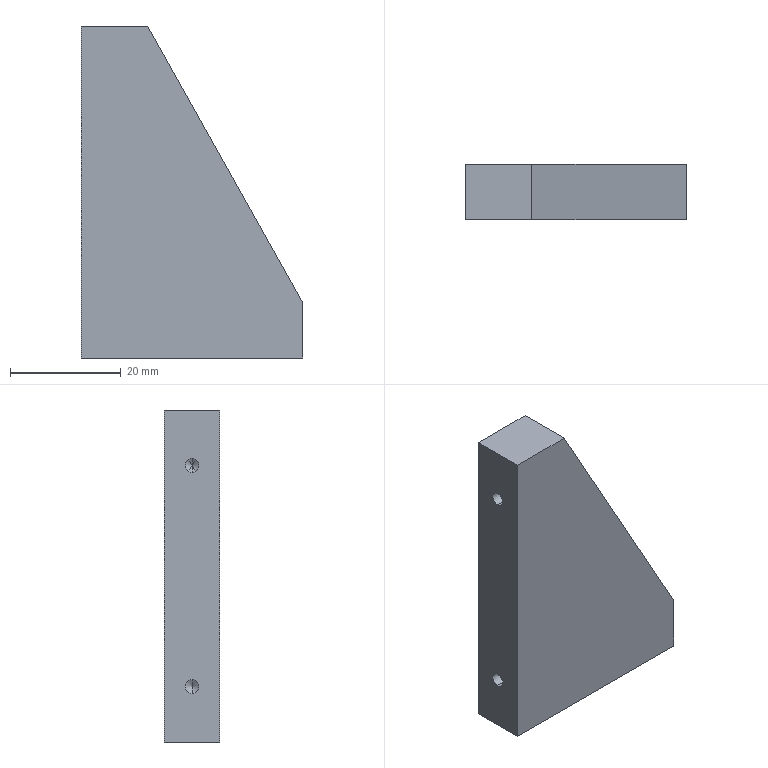Part | STEP file | PN_0031 | 1 solid | 19 faces | box 40 x 10 x 60 mm | volume 16813 mm3 | plane 7 | cylinder 6 | cone 6 | commonest cylinder face diameters 2.5 x4 3.3 x2
STEP:
#1=CARTESIAN_POINT('',(0.,0.,0.));
#2=DIRECTION('',(0.,0.,1.));
#3=DIRECTION('',(1.,0.,0.));
#4=AXIS2_PLACEMENT_3D('',#1,#2,#3);
#5=CARTESIAN_POINT('',(-1.65,5.,-18.5));
#6=VERTEX_POINT('',#5);
#7=CARTESIAN_POINT('',(-1.65,5.,-30.));
#8=VERTEX_POINT('',#7);
#9=CARTESIAN_POINT('',(-1.65,5.,-30.));
#10=DIRECTION('',(0.,0.,-1.));
#11=VECTOR('',#10,1.);
#12=LINE('',#9,#11);
#13=CARTESIAN_POINT('',(0.,5.,-30.));
#14=DIRECTION('',(0.,0.,-1.));
#15=DIRECTION('',(-1.,0.,0.));
#16=AXIS2_PLACEMENT_3D('',#13,#14,#15);
#17=CYLINDRICAL_SURFACE('',#16,1.65);
#18=CARTESIAN_POINT('',(6.283,0.));
#19=DIRECTION('',(0.,1.));
#20=VECTOR('',#19,1.);
#21=LINE('',#18,#20);
#22=(GEOMETRIC_REPRESENTATION_CONTEXT(2)PARAMETRIC_REPRESENTATION_CONTEXT()REPRESENTATION_CONTEXT('',''));
#23=DEFINITIONAL_REPRESENTATION('',(#21),#22);
#24=PCURVE('',#17,#23);
#25=CARTESIAN_POINT('',(0.,5.,-30.));
#26=DIRECTION('',(0.,0.,-1.));
#27=DIRECTION('',(-1.,0.,0.));
#28=AXIS2_PLACEMENT_3D('',#25,#26,#27);
#29=CYLINDRICAL_SURFACE('',#28,1.65);
#30=CARTESIAN_POINT('',(0.,0.));
#31=DIRECTION('',(0.,1.));
#32=VECTOR('',#31,1.);
#33=LINE('',#30,#32);
#34=(GEOMETRIC_REPRESENTATION_CONTEXT(2)PARAMETRIC_REPRESENTATION_CONTEXT()REPRESENTATION_CONTEXT('',''));
#35=DEFINITIONAL_REPRESENTATION('',(#33),#34);
#36=PCURVE('',#29,#35);
#37=SURFACE_CURVE('',#12,(#24,#36),.PCURVE_S1.);
#38=EDGE_CURVE('',#6,#8,#37,.T.);
#39=ORIENTED_EDGE('',*,*,#38,.T.);
#40=CARTESIAN_POINT('',(1.65,5.,-30.));
#41=VERTEX_POINT('',#40);
#42=CARTESIAN_POINT('',(0.,5.,-30.));
#43=DIRECTION('',(0.,0.,-1.));
#44=DIRECTION('',(-1.,0.,0.));
#45=AXIS2_PLACEMENT_3D('',#42,#43,#44);
#46=CIRCLE('',#45,1.65);
#47=CARTESIAN_POINT('',(0.,0.));
#48=DIRECTION('',(1.,0.));
#49=VECTOR('',#48,1.);
#50=LINE('',#47,#49);
#51=(GEOMETRIC_REPRESENTATION_CONTEXT(2)PARAMETRIC_REPRESENTATION_CONTEXT()REPRESENTATION_CONTEXT('',''));
#52=DEFINITIONAL_REPRESENTATION('',(#50),#51);
#53=PCURVE('',#17,#52);
#54=CARTESIAN_POINT('',(-20.,10.,-30.));
#55=DIRECTION('',(0.,0.,1.));
#56=DIRECTION('',(1.,0.,0.));
#57=AXIS2_PLACEMENT_3D('',#54,#55,#56);
#58=PLANE('',#57);
#59=CARTESIAN_POINT('',(18.35,-5.));
#60=CARTESIAN_POINT('',(18.35,-2.142));
#61=CARTESIAN_POINT('',(20.825,-3.571));
#62=CARTESIAN_POINT('',(23.3,-5.));
#63=CARTESIAN_POINT('',(20.825,-6.429));
#64=CARTESIAN_POINT('',(18.35,-7.858));
#65=CARTESIAN_POINT('',(18.35,-5.));
#66=(BOUNDED_CURVE()B_SPLINE_CURVE(2,(#59,#60,#61,#62,#63,#64,#65),.UNSPECIFIED.,.T.,.F.)B_SPLINE_CURVE_WITH_KNOTS((1,2,2,2,2,1),(-2.094,0.,2.094,4.189,6.283,8.378),.UNSPECIFIED.)CURVE()GEOMETRIC_REPRESENTATION_ITEM()RATIONAL_B_SPLINE_CURVE((1.,0.5,1.,0.5,1.,0.5,1.))REPRESENTATION_ITEM(''));
#67=(GEOMETRIC_REPRESENTATION_CONTEXT(2)PARAMETRIC_REPRESENTATION_CONTEXT()REPRESENTATION_CONTEXT('',''));
#68=DEFINITIONAL_REPRESENTATION('',(#66),#67);
#69=PCURVE('',#58,#68);
#70=SURFACE_CURVE('',#46,(#53,#69),.PCURVE_S1.);
#71=EDGE_CURVE('',#41,#8,#70,.T.);
#72=ORIENTED_EDGE('',*,*,#71,.F.);
#73=CARTESIAN_POINT('',(1.65,5.,-18.5));
#74=VERTEX_POINT('',#73);
#75=CARTESIAN_POINT('',(1.65,5.,-30.));
#76=DIRECTION('',(0.,0.,-1.));
#77=VECTOR('',#76,1.);
#78=LINE('',#75,#77);
#79=CARTESIAN_POINT('',(3.142,0.));
#80=DIRECTION('',(0.,1.));
#81=VECTOR('',#80,1.);
#82=LINE('',#79,#81);
#83=(GEOMETRIC_REPRESENTATION_CONTEXT(2)PARAMETRIC_REPRESENTATION_CONTEXT()REPRESENTATION_CONTEXT('',''));
#84=DEFINITIONAL_REPRESENTATION('',(#82),#83);
#85=PCURVE('',#17,#84);
#86=CARTESIAN_POINT('',(3.142,0.));
#87=DIRECTION('',(0.,1.));
#88=VECTOR('',#87,1.);
#89=LINE('',#86,#88);
#90=(GEOMETRIC_REPRESENTATION_CONTEXT(2)PARAMETRIC_REPRESENTATION_CONTEXT()REPRESENTATION_CONTEXT('',''));
#91=DEFINITIONAL_REPRESENTATION('',(#89),#90);
#92=PCURVE('',#29,#91);
#93=SURFACE_CURVE('',#78,(#85,#92),.PCURVE_S1.);
#94=EDGE_CURVE('',#74,#41,#93,.T.);
#95=ORIENTED_EDGE('',*,*,#94,.F.);
#96=CARTESIAN_POINT('',(0.,5.,-18.5));
#97=DIRECTION('',(0.,0.,-1.));
#98=DIRECTION('',(-1.,0.,0.));
#99=AXIS2_PLACEMENT_3D('',#96,#97,#98);
#100=CIRCLE('',#99,1.65);
#101=CARTESIAN_POINT('',(0.,-11.5));
#102=DIRECTION('',(1.,0.));
#103=VECTOR('',#102,1.);
#104=LINE('',#101,#103);
#105=(GEOMETRIC_REPRESENTATION_CONTEXT(2)PARAMETRIC_REPRESENTATION_CONTEXT()REPRESENTATION_CONTEXT('',''));
#106=DEFINITIONAL_REPRESENTATION('',(#104),#105);
#107=PCURVE('',#17,#106);
#108=CARTESIAN_POINT('',(0.,5.,-18.5));
#109=DIRECTION('',(0.,0.,-1.));
#110=DIRECTION('',(-1.,0.,0.));
#111=AXIS2_PLACEMENT_3D('',#108,#109,#110);
#112=CONICAL_SURFACE('',#111,1.65,1.03);
#113=CARTESIAN_POINT('',(0.,0.));
#114=DIRECTION('',(1.,0.));
#115=VECTOR('',#114,1.);
#116=LINE('',#113,#115);
#117=(GEOMETRIC_REPRESENTATION_CONTEXT(2)PARAMETRIC_REPRESENTATION_CONTEXT()REPRESENTATION_CONTEXT('',''));
#118=DEFINITIONAL_REPRESENTATION('',(#116),#117);
#119=PCURVE('',#112,#118);
#120=SURFACE_CURVE('',#100,(#107,#119),.PCURVE_S1.);
#121=EDGE_CURVE('',#74,#6,#120,.T.);
#122=ORIENTED_EDGE('',*,*,#121,.T.);
#123=EDGE_LOOP('',(#39,#72,#95,#122));
#124=FACE_BOUND('',#123,.F.);
#125=ADVANCED_FACE('',(#124),#17,.F.);
#126=ORIENTED_EDGE('',*,*,#121,.F.);
#127=CARTESIAN_POINT('',(0.,5.,-17.509));
#128=VERTEX_POINT('',#127);
#129=CARTESIAN_POINT('',(1.65,5.,-18.5));
#130=DIRECTION('',(0.8572,0.,-0.515));
#131=VECTOR('',#130,1.);
#132=LINE('',#129,#131);
#133=CARTESIAN_POINT('',(3.142,-0.9914));
#134=CARTESIAN_POINT('',(3.142,-0.9764));
#135=CARTESIAN_POINT('',(3.142,-0.9464));
#136=CARTESIAN_POINT('',(3.142,-0.9013));
#137=CARTESIAN_POINT('',(3.142,-0.8562));
#138=CARTESIAN_POINT('',(3.142,-0.8112));
#139=CARTESIAN_POINT('',(3.142,-0.7661));
#140=CARTESIAN_POINT('',(3.142,-0.721));
#141=CARTESIAN_POINT('',(3.142,-0.676));
#142=CARTESIAN_POINT('',(3.142,-0.6309));
#143=CARTESIAN_POINT('',(3.142,-0.5858));
#144=CARTESIAN_POINT('',(3.142,-0.5408));
#145=CARTESIAN_POINT('',(3.142,-0.4957));
#146=CARTESIAN_POINT('',(3.142,-0.4506));
#147=CARTESIAN_POINT('',(3.142,-0.4056));
#148=CARTESIAN_POINT('',(3.142,-0.3605));
#149=CARTESIAN_POINT('',(3.142,-0.3155));
#150=CARTESIAN_POINT('',(3.142,-0.2704));
#151=CARTESIAN_POINT('',(3.142,-0.2253));
#152=CARTESIAN_POINT('',(3.142,-0.1803));
#153=CARTESIAN_POINT('',(3.142,-0.1352));
#154=CARTESIAN_POINT('',(3.142,-0.09013));
#155=CARTESIAN_POINT('',(3.142,-0.04506));
#156=CARTESIAN_POINT('',(3.142,-0.01502));
#157=CARTESIAN_POINT('',(3.142,0.));
#158=B_SPLINE_CURVE_WITH_KNOTS('',3,(#133,#134,#135,#136,#137,#138,#139,#140,#141,#142,#143,#144,#145,#146,#147,#148,#149,#150,#151,#152,#153,#154,#155,#156,#157),.UNSPECIFIED.,.F.,.F.,(4,1,1,1,1,1,1,1,1,1,1,1,1,1,1,1,1,1,1,1,1,1,4),(-1.925,-1.837,-1.75,-1.662,-1.575,-1.487,-1.4,-1.312,-1.225,-1.137,-1.05,-0.9625,-0.875,-0.7875,-0.7,-0.6125,-0.525,-0.4375,-0.35,-0.2625,-0.175,-0.0875,0.),.QUASI_UNIFORM_KNOTS.);
#159=(GEOMETRIC_REPRESENTATION_CONTEXT(2)PARAMETRIC_REPRESENTATION_CONTEXT()REPRESENTATION_CONTEXT('',''));
#160=DEFINITIONAL_REPRESENTATION('',(#158),#159);
#161=PCURVE('',#112,#160);
#162=CARTESIAN_POINT('',(0.,5.,-18.5));
#163=DIRECTION('',(0.,0.,-1.));
#164=DIRECTION('',(-1.,0.,0.));
#165=AXIS2_PLACEMENT_3D('',#162,#163,#164);
#166=CONICAL_SURFACE('',#165,1.65,1.03);
#167=CARTESIAN_POINT('',(3.142,-0.9914));
#168=CARTESIAN_POINT('',(3.142,-0.9764));
#169=CARTESIAN_POINT('',(3.142,-0.9464));
#170=CARTESIAN_POINT('',(3.142,-0.9013));
#171=CARTESIAN_POINT('',(3.142,-0.8562));
#172=CARTESIAN_POINT('',(3.142,-0.8112));
#173=CARTESIAN_POINT('',(3.142,-0.7661));
#174=CARTESIAN_POINT('',(3.142,-0.721));
#175=CARTESIAN_POINT('',(3.142,-0.676));
#176=CARTESIAN_POINT('',(3.142,-0.6309));
#177=CARTESIAN_POINT('',(3.142,-0.5858));
#178=CARTESIAN_POINT('',(3.142,-0.5408));
#179=CARTESIAN_POINT('',(3.142,-0.4957));
#180=CARTESIAN_POINT('',(3.142,-0.4506));
#181=CARTESIAN_POINT('',(3.142,-0.4056));
#182=CARTESIAN_POINT('',(3.142,-0.3605));
#183=CARTESIAN_POINT('',(3.142,-0.3155));
#184=CARTESIAN_POINT('',(3.142,-0.2704));
#185=CARTESIAN_POINT('',(3.142,-0.2253));
#186=CARTESIAN_POINT('',(3.142,-0.1803));
#187=CARTESIAN_POINT('',(3.142,-0.1352));
#188=CARTESIAN_POINT('',(3.142,-0.09013));
#189=CARTESIAN_POINT('',(3.142,-0.04506));
#190=CARTESIAN_POINT('',(3.142,-0.01502));
#191=CARTESIAN_POINT('',(3.142,0.));
#192=B_SPLINE_CURVE_WITH_KNOTS('',3,(#167,#168,#169,#170,#171,#172,#173,#174,#175,#176,#177,#178,#179,#180,#181,#182,#183,#184,#185,#186,#187,#188,#189,#190,#191),.UNSPECIFIED.,.F.,.F.,(4,1,1,1,1,1,1,1,1,1,1,1,1,1,1,1,1,1,1,1,1,1,4),(-1.925,-1.837,-1.75,-1.662,-1.575,-1.487,-1.4,-1.312,-1.225,-1.137,-1.05,-0.9625,-0.875,-0.7875,-0.7,-0.6125,-0.525,-0.4375,-0.35,-0.2625,-0.175,-0.0875,0.),.QUASI_UNIFORM_KNOTS.);
#193=(GEOMETRIC_REPRESENTATION_CONTEXT(2)PARAMETRIC_REPRESENTATION_CONTEXT()REPRESENTATION_CONTEXT('',''));
#194=DEFINITIONAL_REPRESENTATION('',(#192),#193);
#195=PCURVE('',#166,#194);
#196=SURFACE_CURVE('',#132,(#161,#195),.PCURVE_S1.);
#197=EDGE_CURVE('',#128,#74,#196,.T.);
#198=ORIENTED_EDGE('',*,*,#197,.F.);
#199=CARTESIAN_POINT('',(-1.65,5.,-18.5));
#200=DIRECTION('',(-0.8572,0.,-0.515));
#201=VECTOR('',#200,1.);
#202=LINE('',#199,#201);
#203=CARTESIAN_POINT('',(6.283,0.));
#204=DIRECTION('',(0.,1.));
#205=VECTOR('',#204,1.);
#206=LINE('',#203,#205);
#207=(GEOMETRIC_REPRESENTATION_CONTEXT(2)PARAMETRIC_REPRESENTATION_CONTEXT()REPRESENTATION_CONTEXT('',''));
#208=DEFINITIONAL_REPRESENTATION('',(#206),#207);
#209=PCURVE('',#112,#208);
#210=CARTESIAN_POINT('',(0.,0.));
#211=DIRECTION('',(0.,1.));
#212=VECTOR('',#211,1.);
#213=LINE('',#210,#212);
#214=(GEOMETRIC_REPRESENTATION_CONTEXT(2)PARAMETRIC_REPRESENTATION_CONTEXT()REPRESENTATION_CONTEXT('',''));
#215=DEFINITIONAL_REPRESENTATION('',(#213),#214);
#216=PCURVE('',#166,#215);
#217=SURFACE_CURVE('',#202,(#209,#216),.PCURVE_S1.);
#218=EDGE_CURVE('',#128,#6,#217,.T.);
#219=ORIENTED_EDGE('',*,*,#218,.T.);
#220=EDGE_LOOP('',(#126,#198,#219));
#221=FACE_BOUND('',#220,.F.);
#222=ADVANCED_FACE('',(#221),#112,.F.);
#223=CARTESIAN_POINT('',(-11.5,5.,-18.75));
#224=VERTEX_POINT('',#223);
#225=CARTESIAN_POINT('',(-20.,5.,-18.75));
#226=VERTEX_POINT('',#225);
#227=CARTESIAN_POINT('',(-20.,5.,-18.75));
#228=DIRECTION('',(-1.,0.,0.));
#229=VECTOR('',#228,1.);
#230=LINE('',#227,#229);
#231=CARTESIAN_POINT('',(-20.,5.,-20.));
#232=DIRECTION('',(-1.,0.,0.));
#233=DIRECTION('',(0.,0.,1.));
#234=AXIS2_PLACEMENT_3D('',#231,#232,#233);
#235=CYLINDRICAL_SURFACE('',#234,1.25);
#236=CARTESIAN_POINT('',(6.283,0.));
#237=DIRECTION('',(0.,1.));
#238=VECTOR('',#237,1.);
#239=LINE('',#236,#238);
#240=(GEOMETRIC_REPRESENTATION_CONTEXT(2)PARAMETRIC_REPRESENTATION_CONTEXT()REPRESENTATION_CONTEXT('',''));
#241=DEFINITIONAL_REPRESENTATION('',(#239),#240);
#242=PCURVE('',#235,#241);
#243=CARTESIAN_POINT('',(-20.,5.,-20.));
#244=DIRECTION('',(-1.,0.,0.));
#245=DIRECTION('',(0.,0.,1.));
#246=AXIS2_PLACEMENT_3D('',#243,#244,#245);
#247=CYLINDRICAL_SURFACE('',#246,1.25);
#248=CARTESIAN_POINT('',(0.,0.));
#249=DIRECTION('',(0.,1.));
#250=VECTOR('',#249,1.);
#251=LINE('',#248,#250);
#252=(GEOMETRIC_REPRESENTATION_CONTEXT(2)PARAMETRIC_REPRESENTATION_CONTEXT()REPRESENTATION_CONTEXT('',''));
#253=DEFINITIONAL_REPRESENTATION('',(#251),#252);
#254=PCURVE('',#247,#253);
#255=SURFACE_CURVE('',#230,(#242,#254),.PCURVE_S1.);
#256=EDGE_CURVE('',#224,#226,#255,.T.);
#257=ORIENTED_EDGE('',*,*,#256,.T.);
#258=CARTESIAN_POINT('',(-20.,5.,-21.25));
#259=VERTEX_POINT('',#258);
#260=CARTESIAN_POINT('',(-20.,5.,-20.));
#261=DIRECTION('',(-1.,0.,0.));
#262=DIRECTION('',(0.,0.,1.));
#263=AXIS2_PLACEMENT_3D('',#260,#261,#262);
#264=CIRCLE('',#263,1.25);
#265=CARTESIAN_POINT('',(0.,0.));
#266=DIRECTION('',(1.,0.));
#267=VECTOR('',#266,1.);
#268=LINE('',#265,#267);
#269=(GEOMETRIC_REPRESENTATION_CONTEXT(2)PARAMETRIC_REPRESENTATION_CONTEXT()REPRESENTATION_CONTEXT('',''));
#270=DEFINITIONAL_REPRESENTATION('',(#268),#269);
#271=PCURVE('',#235,#270);
#272=CARTESIAN_POINT('',(-20.,10.,30.));
#273=DIRECTION('',(1.,0.,0.));
#274=DIRECTION('',(0.,0.,-1.));
#275=AXIS2_PLACEMENT_3D('',#272,#273,#274);
#276=PLANE('',#275);
#277=CARTESIAN_POINT('',(48.75,-5.));
#278=CARTESIAN_POINT('',(48.75,-2.835));
#279=CARTESIAN_POINT('',(50.625,-3.917));
#280=CARTESIAN_POINT('',(52.5,-5.));
#281=CARTESIAN_POINT('',(50.625,-6.083));
#282=CARTESIAN_POINT('',(48.75,-7.165));
#283=CARTESIAN_POINT('',(48.75,-5.));
#284=(BOUNDED_CURVE()B_SPLINE_CURVE(2,(#277,#278,#279,#280,#281,#282,#283),.UNSPECIFIED.,.T.,.F.)B_SPLINE_CURVE_WITH_KNOTS((1,2,2,2,2,1),(-2.094,0.,2.094,4.189,6.283,8.378),.UNSPECIFIED.)CURVE()GEOMETRIC_REPRESENTATION_ITEM()RATIONAL_B_SPLINE_CURVE((1.,0.5,1.,0.5,1.,0.5,1.))REPRESENTATION_ITEM(''));
#285=(GEOMETRIC_REPRESENTATION_CONTEXT(2)PARAMETRIC_REPRESENTATION_CONTEXT()REPRESENTATION_CONTEXT('',''));
#286=DEFINITIONAL_REPRESENTATION('',(#284),#285);
#287=PCURVE('',#276,#286);
#288=SURFACE_CURVE('',#264,(#271,#287),.PCURVE_S1.);
#289=EDGE_CURVE('',#259,#226,#288,.T.);
#290=ORIENTED_EDGE('',*,*,#289,.F.);
#291=CARTESIAN_POINT('',(-11.5,5.,-21.25));
#292=VERTEX_POINT('',#291);
#293=CARTESIAN_POINT('',(-20.,5.,-21.25));
#294=DIRECTION('',(-1.,0.,0.));
#295=VECTOR('',#294,1.);
#296=LINE('',#293,#295);
#297=CARTESIAN_POINT('',(3.142,0.));
#298=DIRECTION('',(0.,1.));
#299=VECTOR('',#298,1.);
#300=LINE('',#297,#299);
#301=(GEOMETRIC_REPRESENTATION_CONTEXT(2)PARAMETRIC_REPRESENTATION_CONTEXT()REPRESENTATION_CONTEXT('',''));
#302=DEFINITIONAL_REPRESENTATION('',(#300),#301);
#303=PCURVE('',#235,#302);
#304=CARTESIAN_POINT('',(3.142,0.));
#305=DIRECTION('',(0.,1.));
#306=VECTOR('',#305,1.);
#307=LINE('',#304,#306);
#308=(GEOMETRIC_REPRESENTATION_CONTEXT(2)PARAMETRIC_REPRESENTATION_CONTEXT()REPRESENTATION_CONTEXT('',''));
#309=DEFINITIONAL_REPRESENTATION('',(#307),#308);
#310=PCURVE('',#247,#309);
#311=SURFACE_CURVE('',#296,(#303,#310),.PCURVE_S1.);
#312=EDGE_CURVE('',#292,#259,#311,.T.);
#313=ORIENTED_EDGE('',*,*,#312,.F.);
#314=CARTESIAN_POINT('',(-11.5,5.,-20.));
#315=DIRECTION('',(-1.,0.,0.));
#316=DIRECTION('',(0.,0.,1.));
#317=AXIS2_PLACEMENT_3D('',#314,#315,#316);
#318=CIRCLE('',#317,1.25);
#319=CARTESIAN_POINT('',(0.,-8.5));
#320=DIRECTION('',(1.,0.));
#321=VECTOR('',#320,1.);
#322=LINE('',#319,#321);
#323=(GEOMETRIC_REPRESENTATION_CONTEXT(2)PARAMETRIC_REPRESENTATION_CONTEXT()REPRESENTATION_CONTEXT('',''));
#324=DEFINITIONAL_REPRESENTATION('',(#322),#323);
#325=PCURVE('',#235,#324);
#326=CARTESIAN_POINT('',(-11.5,5.,-20.));
#327=DIRECTION('',(-1.,0.,0.));
#328=DIRECTION('',(0.,0.,1.));
#329=AXIS2_PLACEMENT_3D('',#326,#327,#328);
#330=CONICAL_SURFACE('',#329,1.25,1.03);
#331=CARTESIAN_POINT('',(0.,0.));
#332=DIRECTION('',(1.,0.));
#333=VECTOR('',#332,1.);
#334=LINE('',#331,#333);
#335=(GEOMETRIC_REPRESENTATION_CONTEXT(2)PARAMETRIC_REPRESENTATION_CONTEXT()REPRESENTATION_CONTEXT('',''));
#336=DEFINITIONAL_REPRESENTATION('',(#334),#335);
#337=PCURVE('',#330,#336);
#338=SURFACE_CURVE('',#318,(#325,#337),.PCURVE_S1.);
#339=EDGE_CURVE('',#292,#224,#338,.T.);
#340=ORIENTED_EDGE('',*,*,#339,.T.);
#341=EDGE_LOOP('',(#257,#290,#313,#340));
#342=FACE_BOUND('',#341,.F.);
#343=ADVANCED_FACE('',(#342),#235,.F.);
#344=ORIENTED_EDGE('',*,*,#339,.F.);
#345=CARTESIAN_POINT('',(-10.749,5.,-20.));
#346=VERTEX_POINT('',#345);
#347=CARTESIAN_POINT('',(-11.5,5.,-21.25));
#348=DIRECTION('',(-0.515,0.,-0.8572));
#349=VECTOR('',#348,1.);
#350=LINE('',#347,#349);
#351=CARTESIAN_POINT('',(3.142,-0.7511));
#352=CARTESIAN_POINT('',(3.142,-0.7397));
#353=CARTESIAN_POINT('',(3.142,-0.7169));
#354=CARTESIAN_POINT('',(3.142,-0.6828));
#355=CARTESIAN_POINT('',(3.142,-0.6487));
#356=CARTESIAN_POINT('',(3.142,-0.6145));
#357=CARTESIAN_POINT('',(3.142,-0.5804));
#358=CARTESIAN_POINT('',(3.142,-0.5462));
#359=CARTESIAN_POINT('',(3.142,-0.5121));
#360=CARTESIAN_POINT('',(3.142,-0.478));
#361=CARTESIAN_POINT('',(3.142,-0.4438));
#362=CARTESIAN_POINT('',(3.142,-0.4097));
#363=CARTESIAN_POINT('',(3.142,-0.3755));
#364=CARTESIAN_POINT('',(3.142,-0.3414));
#365=CARTESIAN_POINT('',(3.142,-0.3073));
#366=CARTESIAN_POINT('',(3.142,-0.2731));
#367=CARTESIAN_POINT('',(3.142,-0.239));
#368=CARTESIAN_POINT('',(3.142,-0.2048));
#369=CARTESIAN_POINT('',(3.142,-0.1707));
#370=CARTESIAN_POINT('',(3.142,-0.1366));
#371=CARTESIAN_POINT('',(3.142,-0.1024));
#372=CARTESIAN_POINT('',(3.142,-0.06828));
#373=CARTESIAN_POINT('',(3.142,-0.03414));
#374=CARTESIAN_POINT('',(3.142,-0.01138));
#375=CARTESIAN_POINT('',(3.142,0.));
#376=B_SPLINE_CURVE_WITH_KNOTS('',3,(#351,#352,#353,#354,#355,#356,#357,#358,#359,#360,#361,#362,#363,#364,#365,#366,#367,#368,#369,#370,#371,#372,#373,#374,#375),.UNSPECIFIED.,.F.,.F.,(4,1,1,1,1,1,1,1,1,1,1,1,1,1,1,1,1,1,1,1,1,1,4),(-1.458,-1.392,-1.326,-1.259,-1.193,-1.127,-1.061,-0.9943,-0.928,-0.8617,-0.7954,-0.7291,-0.6629,-0.5966,-0.5303,-0.464,-0.3977,-0.3314,-0.2651,-0.1989,-0.1326,-0.06629,0.),.QUASI_UNIFORM_KNOTS.);
#377=(GEOMETRIC_REPRESENTATION_CONTEXT(2)PARAMETRIC_REPRESENTATION_CONTEXT()REPRESENTATION_CONTEXT('',''));
#378=DEFINITIONAL_REPRESENTATION('',(#376),#377);
#379=PCURVE('',#330,#378);
#380=CARTESIAN_POINT('',(-11.5,5.,-20.));
#381=DIRECTION('',(-1.,0.,0.));
#382=DIRECTION('',(0.,0.,1.));
#383=AXIS2_PLACEMENT_3D('',#380,#381,#382);
#384=CONICAL_SURFACE('',#383,1.25,1.03);
#385=CARTESIAN_POINT('',(3.142,-0.7511));
#386=CARTESIAN_POINT('',(3.142,-0.7397));
#387=CARTESIAN_POINT('',(3.142,-0.7169));
#388=CARTESIAN_POINT('',(3.142,-0.6828));
#389=CARTESIAN_POINT('',(3.142,-0.6487));
#390=CARTESIAN_POINT('',(3.142,-0.6145));
#391=CARTESIAN_POINT('',(3.142,-0.5804));
#392=CARTESIAN_POINT('',(3.142,-0.5462));
#393=CARTESIAN_POINT('',(3.142,-0.5121));
#394=CARTESIAN_POINT('',(3.142,-0.478));
#395=CARTESIAN_POINT('',(3.142,-0.4438));
#396=CARTESIAN_POINT('',(3.142,-0.4097));
#397=CARTESIAN_POINT('',(3.142,-0.3755));
#398=CARTESIAN_POINT('',(3.142,-0.3414));
#399=CARTESIAN_POINT('',(3.142,-0.3073));
#400=CARTESIAN_POINT('',(3.142,-0.2731));
#401=CARTESIAN_POINT('',(3.142,-0.239));
#402=CARTESIAN_POINT('',(3.142,-0.2048));
#403=CARTESIAN_POINT('',(3.142,-0.1707));
#404=CARTESIAN_POINT('',(3.142,-0.1366));
#405=CARTESIAN_POINT('',(3.142,-0.1024));
#406=CARTESIAN_POINT('',(3.142,-0.06828));
#407=CARTESIAN_POINT('',(3.142,-0.03414));
#408=CARTESIAN_POINT('',(3.142,-0.01138));
#409=CARTESIAN_POINT('',(3.142,0.));
#410=B_SPLINE_CURVE_WITH_KNOTS('',3,(#385,#386,#387,#388,#389,#390,#391,#392,#393,#394,#395,#396,#397,#398,#399,#400,#401,#402,#403,#404,#405,#406,#407,#408,#409),.UNSPECIFIED.,.F.,.F.,(4,1,1,1,1,1,1,1,1,1,1,1,1,1,1,1,1,1,1,1,1,1,4),(-1.458,-1.392,-1.326,-1.259,-1.193,-1.127,-1.061,-0.9943,-0.928,-0.8617,-0.7954,-0.7291,-0.6629,-0.5966,-0.5303,-0.464,-0.3977,-0.3314,-0.2651,-0.1989,-0.1326,-0.06629,0.),.QUASI_UNIFORM_KNOTS.);
#411=(GEOMETRIC_REPRESENTATION_CONTEXT(2)PARAMETRIC_REPRESENTATION_CONTEXT()REPRESENTATION_CONTEXT('',''));
#412=DEFINITIONAL_REPRESENTATION('',(#410),#411);
#413=PCURVE('',#384,#412);
#414=SURFACE_CURVE('',#350,(#379,#413),.PCURVE_S1.);
#415=EDGE_CURVE('',#346,#292,#414,.T.);
#416=ORIENTED_EDGE('',*,*,#415,.F.);
#417=CARTESIAN_POINT('',(-11.5,5.,-18.75));
#418=DIRECTION('',(-0.515,0.,0.8572));
#419=VECTOR('',#418,1.);
#420=LINE('',#417,#419);
#421=CARTESIAN_POINT('',(6.283,0.));
#422=DIRECTION('',(0.,1.));
#423=VECTOR('',#422,1.);
#424=LINE('',#421,#423);
#425=(GEOMETRIC_REPRESENTATION_CONTEXT(2)PARAMETRIC_REPRESENTATION_CONTEXT()REPRESENTATION_CONTEXT('',''));
#426=DEFINITIONAL_REPRESENTATION('',(#424),#425);
#427=PCURVE('',#330,#426);
#428=CARTESIAN_POINT('',(0.,0.));
#429=DIRECTION('',(0.,1.));
#430=VECTOR('',#429,1.);
#431=LINE('',#428,#430);
#432=(GEOMETRIC_REPRESENTATION_CONTEXT(2)PARAMETRIC_REPRESENTATION_CONTEXT()REPRESENTATION_CONTEXT('',''));
#433=DEFINITIONAL_REPRESENTATION('',(#431),#432);
#434=PCURVE('',#384,#433);
#435=SURFACE_CURVE('',#420,(#427,#434),.PCURVE_S1.);
#436=EDGE_CURVE('',#346,#224,#435,.T.);
#437=ORIENTED_EDGE('',*,*,#436,.T.);
#438=EDGE_LOOP('',(#344,#416,#437));
#439=FACE_BOUND('',#438,.F.);
#440=ADVANCED_FACE('',(#439),#330,.F.);
#441=CARTESIAN_POINT('',(-11.5,5.,21.25));
#442=VERTEX_POINT('',#441);
#443=CARTESIAN_POINT('',(-20.,5.,21.25));
#444=VERTEX_POINT('',#443);
#445=CARTESIAN_POINT('',(-20.,5.,21.25));
#446=DIRECTION('',(-1.,0.,0.));
#447=VECTOR('',#446,1.);
#448=LINE('',#445,#447);
#449=CARTESIAN_POINT('',(-20.,5.,20.));
#450=DIRECTION('',(-1.,0.,0.));
#451=DIRECTION('',(0.,0.,1.));
#452=AXIS2_PLACEMENT_3D('',#449,#450,#451);
#453=CYLINDRICAL_SURFACE('',#452,1.25);
#454=CARTESIAN_POINT('',(6.283,0.));
#455=DIRECTION('',(0.,1.));
#456=VECTOR('',#455,1.);
#457=LINE('',#454,#456);
#458=(GEOMETRIC_REPRESENTATION_CONTEXT(2)PARAMETRIC_REPRESENTATION_CONTEXT()REPRESENTATION_CONTEXT('',''));
#459=DEFINITIONAL_REPRESENTATION('',(#457),#458);
#460=PCURVE('',#453,#459);
#461=CARTESIAN_POINT('',(-20.,5.,20.));
#462=DIRECTION('',(-1.,0.,0.));
#463=DIRECTION('',(0.,0.,1.));
#464=AXIS2_PLACEMENT_3D('',#461,#462,#463);
#465=CYLINDRICAL_SURFACE('',#464,1.25);
#466=CARTESIAN_POINT('',(0.,0.));
#467=DIRECTION('',(0.,1.));
#468=VECTOR('',#467,1.);
#469=LINE('',#466,#468);
#470=(GEOMETRIC_REPRESENTATION_CONTEXT(2)PARAMETRIC_REPRESENTATION_CONTEXT()REPRESENTATION_CONTEXT('',''));
#471=DEFINITIONAL_REPRESENTATION('',(#469),#470);
#472=PCURVE('',#465,#471);
#473=SURFACE_CURVE('',#448,(#460,#472),.PCURVE_S1.);
#474=EDGE_CURVE('',#442,#444,#473,.T.);
#475=ORIENTED_EDGE('',*,*,#474,.T.);
#476=CARTESIAN_POINT('',(-20.,5.,18.75));
#477=VERTEX_POINT('',#476);
#478=CARTESIAN_POINT('',(-20.,5.,20.));
#479=DIRECTION('',(-1.,0.,0.));
#480=DIRECTION('',(0.,0.,1.));
#481=AXIS2_PLACEMENT_3D('',#478,#479,#480);
#482=CIRCLE('',#481,1.25);
#483=CARTESIAN_POINT('',(0.,0.));
#484=DIRECTION('',(1.,0.));
#485=VECTOR('',#484,1.);
#486=LINE('',#483,#485);
#487=(GEOMETRIC_REPRESENTATION_CONTEXT(2)PARAMETRIC_REPRESENTATION_CONTEXT()REPRESENTATION_CONTEXT('',''));
#488=DEFINITIONAL_REPRESENTATION('',(#486),#487);
#489=PCURVE('',#453,#488);
#490=CARTESIAN_POINT('',(8.75,-5.));
#491=CARTESIAN_POINT('',(8.75,-2.835));
#492=CARTESIAN_POINT('',(10.625,-3.917));
#493=CARTESIAN_POINT('',(12.5,-5.));
#494=CARTESIAN_POINT('',(10.625,-6.083));
#495=CARTESIAN_POINT('',(8.75,-7.165));
#496=CARTESIAN_POINT('',(8.75,-5.));
#497=(BOUNDED_CURVE()B_SPLINE_CURVE(2,(#490,#491,#492,#493,#494,#495,#496),.UNSPECIFIED.,.T.,.F.)B_SPLINE_CURVE_WITH_KNOTS((1,2,2,2,2,1),(-2.094,0.,2.094,4.189,6.283,8.378),.UNSPECIFIED.)CURVE()GEOMETRIC_REPRESENTATION_ITEM()RATIONAL_B_SPLINE_CURVE((1.,0.5,1.,0.5,1.,0.5,1.))REPRESENTATION_ITEM(''));
#498=(GEOMETRIC_REPRESENTATION_CONTEXT(2)PARAMETRIC_REPRESENTATION_CONTEXT()REPRESENTATION_CONTEXT('',''));
#499=DEFINITIONAL_REPRESENTATION('',(#497),#498);
#500=PCURVE('',#276,#499);
#501=SURFACE_CURVE('',#482,(#489,#500),.PCURVE_S1.);
#502=EDGE_CURVE('',#477,#444,#501,.T.);
#503=ORIENTED_EDGE('',*,*,#502,.F.);
#504=CARTESIAN_POINT('',(-11.5,5.,18.75));
#505=VERTEX_POINT('',#504);
#506=CARTESIAN_POINT('',(-20.,5.,18.75));
#507=DIRECTION('',(-1.,0.,0.));
#508=VECTOR('',#507,1.);
#509=LINE('',#506,#508);
#510=CARTESIAN_POINT('',(3.142,0.));
#511=DIRECTION('',(0.,1.));
#512=VECTOR('',#511,1.);
#513=LINE('',#510,#512);
#514=(GEOMETRIC_REPRESENTATION_CONTEXT(2)PARAMETRIC_REPRESENTATION_CONTEXT()REPRESENTATION_CONTEXT('',''));
#515=DEFINITIONAL_REPRESENTATION('',(#513),#514);
#516=PCURVE('',#453,#515);
#517=CARTESIAN_POINT('',(3.142,0.));
#518=DIRECTION('',(0.,1.));
#519=VECTOR('',#518,1.);
#520=LINE('',#517,#519);
#521=(GEOMETRIC_REPRESENTATION_CONTEXT(2)PARAMETRIC_REPRESENTATION_CONTEXT()REPRESENTATION_CONTEXT('',''));
#522=DEFINITIONAL_REPRESENTATION('',(#520),#521);
#523=PCURVE('',#465,#522);
#524=SURFACE_CURVE('',#509,(#516,#523),.PCURVE_S1.);
#525=EDGE_CURVE('',#505,#477,#524,.T.);
#526=ORIENTED_EDGE('',*,*,#525,.F.);
#527=CARTESIAN_POINT('',(-11.5,5.,20.));
#528=DIRECTION('',(-1.,0.,0.));
#529=DIRECTION('',(0.,0.,1.));
#530=AXIS2_PLACEMENT_3D('',#527,#528,#529);
#531=CIRCLE('',#530,1.25);
#532=CARTESIAN_POINT('',(0.,-8.5));
#533=DIRECTION('',(1.,0.));
#534=VECTOR('',#533,1.);
#535=LINE('',#532,#534);
#536=(GEOMETRIC_REPRESENTATION_CONTEXT(2)PARAMETRIC_REPRESENTATION_CONTEXT()REPRESENTATION_CONTEXT('',''));
#537=DEFINITIONAL_REPRESENTATION('',(#535),#536);
#538=PCURVE('',#453,#537);
#539=CARTESIAN_POINT('',(-11.5,5.,20.));
#540=DIRECTION('',(-1.,0.,0.));
#541=DIRECTION('',(0.,0.,1.));
#542=AXIS2_PLACEMENT_3D('',#539,#540,#541);
#543=CONICAL_SURFACE('',#542,1.25,1.03);
#544=CARTESIAN_POINT('',(0.,0.));
#545=DIRECTION('',(1.,0.));
#546=VECTOR('',#545,1.);
#547=LINE('',#544,#546);
#548=(GEOMETRIC_REPRESENTATION_CONTEXT(2)PARAMETRIC_REPRESENTATION_CONTEXT()REPRESENTATION_CONTEXT('',''));
#549=DEFINITIONAL_REPRESENTATION('',(#547),#548);
#550=PCURVE('',#543,#549);
#551=SURFACE_CURVE('',#531,(#538,#550),.PCURVE_S1.);
#552=EDGE_CURVE('',#505,#442,#551,.T.);
#553=ORIENTED_EDGE('',*,*,#552,.T.);
#554=EDGE_LOOP('',(#475,#503,#526,#553));
#555=FACE_BOUND('',#554,.F.);
#556=ADVANCED_FACE('',(#555),#453,.F.);
#557=ORIENTED_EDGE('',*,*,#552,.F.);
#558=CARTESIAN_POINT('',(-10.749,5.,20.));
#559=VERTEX_POINT('',#558);
#560=CARTESIAN_POINT('',(-11.5,5.,18.75));
#561=DIRECTION('',(-0.515,0.,-0.8572));
#562=VECTOR('',#561,1.);
#563=LINE('',#560,#562);
#564=CARTESIAN_POINT('',(3.142,-0.7511));
#565=CARTESIAN_POINT('',(3.142,-0.7397));
#566=CARTESIAN_POINT('',(3.142,-0.7169));
#567=CARTESIAN_POINT('',(3.142,-0.6828));
#568=CARTESIAN_POINT('',(3.142,-0.6487));
#569=CARTESIAN_POINT('',(3.142,-0.6145));
#570=CARTESIAN_POINT('',(3.142,-0.5804));
#571=CARTESIAN_POINT('',(3.142,-0.5462));
#572=CARTESIAN_POINT('',(3.142,-0.5121));
#573=CARTESIAN_POINT('',(3.142,-0.478));
#574=CARTESIAN_POINT('',(3.142,-0.4438));
#575=CARTESIAN_POINT('',(3.142,-0.4097));
#576=CARTESIAN_POINT('',(3.142,-0.3755));
#577=CARTESIAN_POINT('',(3.142,-0.3414));
#578=CARTESIAN_POINT('',(3.142,-0.3073));
#579=CARTESIAN_POINT('',(3.142,-0.2731));
#580=CARTESIAN_POINT('',(3.142,-0.239));
#581=CARTESIAN_POINT('',(3.142,-0.2048));
#582=CARTESIAN_POINT('',(3.142,-0.1707));
#583=CARTESIAN_POINT('',(3.142,-0.1366));
#584=CARTESIAN_POINT('',(3.142,-0.1024));
#585=CARTESIAN_POINT('',(3.142,-0.06828));
#586=CARTESIAN_POINT('',(3.142,-0.03414));
#587=CARTESIAN_POINT('',(3.142,-0.01138));
#588=CARTESIAN_POINT('',(3.142,0.));
#589=B_SPLINE_CURVE_WITH_KNOTS('',3,(#564,#565,#566,#567,#568,#569,#570,#571,#572,#573,#574,#575,#576,#577,#578,#579,#580,#581,#582,#583,#584,#585,#586,#587,#588),.UNSPECIFIED.,.F.,.F.,(4,1,1,1,1,1,1,1,1,1,1,1,1,1,1,1,1,1,1,1,1,1,4),(-1.458,-1.392,-1.326,-1.259,-1.193,-1.127,-1.061,-0.9943,-0.928,-0.8617,-0.7954,-0.7291,-0.6629,-0.5966,-0.5303,-0.464,-0.3977,-0.3314,-0.2651,-0.1989,-0.1326,-0.06629,0.),.UNSPECIFIED.);
#590=(GEOMETRIC_REPRESENTATION_CONTEXT(2)PARAMETRIC_REPRESENTATION_CONTEXT()REPRESENTATION_CONTEXT('',''));
#591=DEFINITIONAL_REPRESENTATION('',(#589),#590);
#592=PCURVE('',#543,#591);
#593=CARTESIAN_POINT('',(-11.5,5.,20.));
#594=DIRECTION('',(-1.,0.,0.));
#595=DIRECTION('',(0.,0.,1.));
#596=AXIS2_PLACEMENT_3D('',#593,#594,#595);
#597=CONICAL_SURFACE('',#596,1.25,1.03);
#598=CARTESIAN_POINT('',(3.142,-0.7511));
#599=CARTESIAN_POINT('',(3.142,-0.7397));
#600=CARTESIAN_POINT('',(3.142,-0.7169));
#601=CARTESIAN_POINT('',(3.142,-0.6828));
#602=CARTESIAN_POINT('',(3.142,-0.6487));
#603=CARTESIAN_POINT('',(3.142,-0.6145));
#604=CARTESIAN_POINT('',(3.142,-0.5804));
#605=CARTESIAN_POINT('',(3.142,-0.5462));
#606=CARTESIAN_POINT('',(3.142,-0.5121));
#607=CARTESIAN_POINT('',(3.142,-0.478));
#608=CARTESIAN_POINT('',(3.142,-0.4438));
#609=CARTESIAN_POINT('',(3.142,-0.4097));
#610=CARTESIAN_POINT('',(3.142,-0.3755));
#611=CARTESIAN_POINT('',(3.142,-0.3414));
#612=CARTESIAN_POINT('',(3.142,-0.3073));
#613=CARTESIAN_POINT('',(3.142,-0.2731));
#614=CARTESIAN_POINT('',(3.142,-0.239));
#615=CARTESIAN_POINT('',(3.142,-0.2048));
#616=CARTESIAN_POINT('',(3.142,-0.1707));
#617=CARTESIAN_POINT('',(3.142,-0.1366));
#618=CARTESIAN_POINT('',(3.142,-0.1024));
#619=CARTESIAN_POINT('',(3.142,-0.06828));
#620=CARTESIAN_POINT('',(3.142,-0.03414));
#621=CARTESIAN_POINT('',(3.142,-0.01138));
#622=CARTESIAN_POINT('',(3.142,0.));
#623=B_SPLINE_CURVE_WITH_KNOTS('',3,(#598,#599,#600,#601,#602,#603,#604,#605,#606,#607,#608,#609,#610,#611,#612,#613,#614,#615,#616,#617,#618,#619,#620,#621,#622),.UNSPECIFIED.,.F.,.F.,(4,1,1,1,1,1,1,1,1,1,1,1,1,1,1,1,1,1,1,1,1,1,4),(-1.458,-1.392,-1.326,-1.259,-1.193,-1.127,-1.061,-0.9943,-0.928,-0.8617,-0.7954,-0.7291,-0.6629,-0.5966,-0.5303,-0.464,-0.3977,-0.3314,-0.2651,-0.1989,-0.1326,-0.06629,0.),.UNSPECIFIED.);
#624=(GEOMETRIC_REPRESENTATION_CONTEXT(2)PARAMETRIC_REPRESENTATION_CONTEXT()REPRESENTATION_CONTEXT('',''));
#625=DEFINITIONAL_REPRESENTATION('',(#623),#624);
#626=PCURVE('',#597,#625);
#627=SURFACE_CURVE('',#563,(#592,#626),.PCURVE_S1.);
#628=EDGE_CURVE('',#559,#505,#627,.T.);
#629=ORIENTED_EDGE('',*,*,#628,.F.);
#630=CARTESIAN_POINT('',(-11.5,5.,21.25));
#631=DIRECTION('',(-0.515,0.,0.8572));
#632=VECTOR('',#631,1.);
#633=LINE('',#630,#632);
#634=CARTESIAN_POINT('',(6.283,0.));
#635=DIRECTION('',(0.,1.));
#636=VECTOR('',#635,1.);
#637=LINE('',#634,#636);
#638=(GEOMETRIC_REPRESENTATION_CONTEXT(2)PARAMETRIC_REPRESENTATION_CONTEXT()REPRESENTATION_CONTEXT('',''));
#639=DEFINITIONAL_REPRESENTATION('',(#637),#638);
#640=PCURVE('',#543,#639);
#641=CARTESIAN_POINT('',(0.,0.));
#642=DIRECTION('',(0.,1.));
#643=VECTOR('',#642,1.);
#644=LINE('',#641,#643);
#645=(GEOMETRIC_REPRESENTATION_CONTEXT(2)PARAMETRIC_REPRESENTATION_CONTEXT()REPRESENTATION_CONTEXT('',''));
#646=DEFINITIONAL_REPRESENTATION('',(#644),#645);
#647=PCURVE('',#597,#646);
#648=SURFACE_CURVE('',#633,(#640,#647),.PCURVE_S1.);
#649=EDGE_CURVE('',#559,#442,#648,.T.);
#650=ORIENTED_EDGE('',*,*,#649,.T.);
#651=EDGE_LOOP('',(#557,#629,#650));
#652=FACE_BOUND('',#651,.F.);
#653=ADVANCED_FACE('',(#652),#543,.F.);
#654=CARTESIAN_POINT('',(20.,10.,-20.));
#655=VERTEX_POINT('',#654);
#656=CARTESIAN_POINT('',(20.,10.,-30.));
#657=VERTEX_POINT('',#656);
#658=CARTESIAN_POINT('',(20.,10.,30.));
#659=DIRECTION('',(0.,0.,-1.));
#660=VECTOR('',#659,1.);
#661=LINE('',#658,#660);
#662=CARTESIAN_POINT('',(20.,10.,30.));
#663=DIRECTION('',(-1.,0.,0.));
#664=DIRECTION('',(0.,0.,1.));
#665=AXIS2_PLACEMENT_3D('',#662,#663,#664);
#666=PLANE('',#665);
#667=CARTESIAN_POINT('',(0.,0.));
#668=DIRECTION('',(-1.,0.));
#669=VECTOR('',#668,1.);
#670=LINE('',#667,#669);
#671=(GEOMETRIC_REPRESENTATION_CONTEXT(2)PARAMETRIC_REPRESENTATION_CONTEXT()REPRESENTATION_CONTEXT('',''));
#672=DEFINITIONAL_REPRESENTATION('',(#670),#671);
#673=PCURVE('',#666,#672);
#674=CARTESIAN_POINT('',(0.,10.,0.));
#675=DIRECTION('',(0.,-1.,0.));
#676=DIRECTION('',(0.,0.,-1.));
#677=AXIS2_PLACEMENT_3D('',#674,#675,#676);
#678=PLANE('',#677);
#679=CARTESIAN_POINT('',(-30.,20.));
#680=DIRECTION('',(1.,0.));
#681=VECTOR('',#680,1.);
#682=LINE('',#679,#681);
#683=(GEOMETRIC_REPRESENTATION_CONTEXT(2)PARAMETRIC_REPRESENTATION_CONTEXT()REPRESENTATION_CONTEXT('',''));
#684=DEFINITIONAL_REPRESENTATION('',(#682),#683);
#685=PCURVE('',#678,#684);
#686=SURFACE_CURVE('',#661,(#673,#685),.PCURVE_S1.);
#687=EDGE_CURVE('',#655,#657,#686,.T.);
#688=ORIENTED_EDGE('',*,*,#687,.F.);
#689=CARTESIAN_POINT('',(20.,0.,-20.));
#690=VERTEX_POINT('',#689);
#691=CARTESIAN_POINT('',(20.,10.,-20.));
#692=DIRECTION('',(0.,-1.,0.));
#693=VECTOR('',#692,1.);
#694=LINE('',#691,#693);
#695=CARTESIAN_POINT('',(-50.,0.));
#696=DIRECTION('',(0.,-1.));
#697=VECTOR('',#696,1.);
#698=LINE('',#695,#697);
#699=(GEOMETRIC_REPRESENTATION_CONTEXT(2)PARAMETRIC_REPRESENTATION_CONTEXT()REPRESENTATION_CONTEXT('',''));
#700=DEFINITIONAL_REPRESENTATION('',(#698),#699);
#701=PCURVE('',#666,#700);
#702=CARTESIAN_POINT('',(20.,10.,-20.));
#703=DIRECTION('',(-0.8725,0.,-0.4886));
#704=DIRECTION('',(0.,-1.,0.));
#705=AXIS2_PLACEMENT_3D('',#702,#703,#704);
#706=PLANE('',#705);
#707=CARTESIAN_POINT('',(0.,0.));
#708=DIRECTION('',(1.,0.));
#709=VECTOR('',#708,1.);
#710=LINE('',#707,#709);
#711=(GEOMETRIC_REPRESENTATION_CONTEXT(2)PARAMETRIC_REPRESENTATION_CONTEXT()REPRESENTATION_CONTEXT('',''));
#712=DEFINITIONAL_REPRESENTATION('',(#710),#711);
#713=PCURVE('',#706,#712);
#714=SURFACE_CURVE('',#694,(#701,#713),.PCURVE_S1.);
#715=EDGE_CURVE('',#655,#690,#714,.T.);
#716=ORIENTED_EDGE('',*,*,#715,.T.);
#717=CARTESIAN_POINT('',(20.,0.,-30.));
#718=VERTEX_POINT('',#717);
#719=CARTESIAN_POINT('',(20.,0.,30.));
#720=DIRECTION('',(0.,0.,-1.));
#721=VECTOR('',#720,1.);
#722=LINE('',#719,#721);
#723=CARTESIAN_POINT('',(0.,-10.));
#724=DIRECTION('',(-1.,0.));
#725=VECTOR('',#724,1.);
#726=LINE('',#723,#725);
#727=(GEOMETRIC_REPRESENTATION_CONTEXT(2)PARAMETRIC_REPRESENTATION_CONTEXT()REPRESENTATION_CONTEXT('',''));
#728=DEFINITIONAL_REPRESENTATION('',(#726),#727);
#729=PCURVE('',#666,#728);
#730=CARTESIAN_POINT('',(0.,0.,0.));
#731=DIRECTION('',(0.,-1.,0.));
#732=DIRECTION('',(0.,0.,-1.));
#733=AXIS2_PLACEMENT_3D('',#730,#731,#732);
#734=PLANE('',#733);
#735=CARTESIAN_POINT('',(-30.,20.));
#736=DIRECTION('',(1.,0.));
#737=VECTOR('',#736,1.);
#738=LINE('',#735,#737);
#739=(GEOMETRIC_REPRESENTATION_CONTEXT(2)PARAMETRIC_REPRESENTATION_CONTEXT()REPRESENTATION_CONTEXT('',''));
#740=DEFINITIONAL_REPRESENTATION('',(#738),#739);
#741=PCURVE('',#734,#740);
#742=SURFACE_CURVE('',#722,(#729,#741),.PCURVE_S1.);
#743=EDGE_CURVE('',#690,#718,#742,.T.);
#744=ORIENTED_EDGE('',*,*,#743,.T.);
#745=CARTESIAN_POINT('',(20.,10.,-30.));
#746=DIRECTION('',(0.,-1.,0.));
#747=VECTOR('',#746,1.);
#748=LINE('',#745,#747);
#749=CARTESIAN_POINT('',(-60.,0.));
#750=DIRECTION('',(0.,-1.));
#751=VECTOR('',#750,1.);
#752=LINE('',#749,#751);
#753=(GEOMETRIC_REPRESENTATION_CONTEXT(2)PARAMETRIC_REPRESENTATION_CONTEXT()REPRESENTATION_CONTEXT('',''));
#754=DEFINITIONAL_REPRESENTATION('',(#752),#753);
#755=PCURVE('',#666,#754);
#756=CARTESIAN_POINT('',(40.,0.));
#757=DIRECTION('',(0.,-1.));
#758=VECTOR('',#757,1.);
#759=LINE('',#756,#758);
#760=(GEOMETRIC_REPRESENTATION_CONTEXT(2)PARAMETRIC_REPRESENTATION_CONTEXT()REPRESENTATION_CONTEXT('',''));
#761=DEFINITIONAL_REPRESENTATION('',(#759),#760);
#762=PCURVE('',#58,#761);
#763=SURFACE_CURVE('',#748,(#755,#762),.PCURVE_S1.);
#764=EDGE_CURVE('',#657,#718,#763,.T.);
#765=ORIENTED_EDGE('',*,*,#764,.F.);
#766=EDGE_LOOP('',(#688,#716,#744,#765));
#767=FACE_BOUND('',#766,.T.);
#768=ADVANCED_FACE('',(#767),#666,.F.);
#769=CARTESIAN_POINT('',(0.,5.,-30.));
#770=DIRECTION('',(0.,0.,-1.));
#771=DIRECTION('',(-1.,0.,0.));
#772=AXIS2_PLACEMENT_3D('',#769,#770,#771);
#773=CIRCLE('',#772,1.65);
#774=CARTESIAN_POINT('',(18.35,-5.));
#775=CARTESIAN_POINT('',(18.35,-2.142));
#776=CARTESIAN_POINT('',(20.825,-3.571));
#777=CARTESIAN_POINT('',(23.3,-5.));
#778=CARTESIAN_POINT('',(20.825,-6.429));
#779=CARTESIAN_POINT('',(18.35,-7.858));
#780=CARTESIAN_POINT('',(18.35,-5.));
#781=(BOUNDED_CURVE()B_SPLINE_CURVE(2,(#774,#775,#776,#777,#778,#779,#780),.UNSPECIFIED.,.T.,.F.)B_SPLINE_CURVE_WITH_KNOTS((1,2,2,2,2,1),(-2.094,0.,2.094,4.189,6.283,8.378),.UNSPECIFIED.)CURVE()GEOMETRIC_REPRESENTATION_ITEM()RATIONAL_B_SPLINE_CURVE((1.,0.5,1.,0.5,1.,0.5,1.))REPRESENTATION_ITEM(''));
#782=(GEOMETRIC_REPRESENTATION_CONTEXT(2)PARAMETRIC_REPRESENTATION_CONTEXT()REPRESENTATION_CONTEXT('',''));
#783=DEFINITIONAL_REPRESENTATION('',(#781),#782);
#784=PCURVE('',#58,#783);
#785=CARTESIAN_POINT('',(0.,0.));
#786=DIRECTION('',(1.,0.));
#787=VECTOR('',#786,1.);
#788=LINE('',#785,#787);
#789=(GEOMETRIC_REPRESENTATION_CONTEXT(2)PARAMETRIC_REPRESENTATION_CONTEXT()REPRESENTATION_CONTEXT('',''));
#790=DEFINITIONAL_REPRESENTATION('',(#788),#789);
#791=PCURVE('',#29,#790);
#792=SURFACE_CURVE('',#773,(#784,#791),.PCURVE_S1.);
#793=EDGE_CURVE('',#8,#41,#792,.T.);
#794=ORIENTED_EDGE('',*,*,#793,.F.);
#795=ORIENTED_EDGE('',*,*,#71,.F.);
#796=EDGE_LOOP('',(#794,#795));
#797=FACE_BOUND('',#796,.T.);
#798=CARTESIAN_POINT('',(-20.,0.,-30.));
#799=VERTEX_POINT('',#798);
#800=CARTESIAN_POINT('',(-20.,0.,-30.));
#801=DIRECTION('',(-1.,0.,0.));
#802=VECTOR('',#801,1.);
#803=LINE('',#800,#802);
#804=CARTESIAN_POINT('',(0.,-10.));
#805=DIRECTION('',(-1.,0.));
#806=VECTOR('',#805,1.);
#807=LINE('',#804,#806);
#808=(GEOMETRIC_REPRESENTATION_CONTEXT(2)PARAMETRIC_REPRESENTATION_CONTEXT()REPRESENTATION_CONTEXT('',''));
#809=DEFINITIONAL_REPRESENTATION('',(#807),#808);
#810=PCURVE('',#58,#809);
#811=CARTESIAN_POINT('',(30.,-20.));
#812=DIRECTION('',(0.,-1.));
#813=VECTOR('',#812,1.);
#814=LINE('',#811,#813);
#815=(GEOMETRIC_REPRESENTATION_CONTEXT(2)PARAMETRIC_REPRESENTATION_CONTEXT()REPRESENTATION_CONTEXT('',''));
#816=DEFINITIONAL_REPRESENTATION('',(#814),#815);
#817=PCURVE('',#734,#816);
#818=SURFACE_CURVE('',#803,(#810,#817),.PCURVE_S1.);
#819=EDGE_CURVE('',#718,#799,#818,.T.);
#820=ORIENTED_EDGE('',*,*,#819,.T.);
#821=CARTESIAN_POINT('',(-20.,10.,-30.));
#822=VERTEX_POINT('',#821);
#823=CARTESIAN_POINT('',(-20.,10.,-30.));
#824=DIRECTION('',(0.,-1.,0.));
#825=VECTOR('',#824,1.);
#826=LINE('',#823,#825);
#827=CARTESIAN_POINT('',(0.,0.));
#828=DIRECTION('',(0.,-1.));
#829=VECTOR('',#828,1.);
#830=LINE('',#827,#829);
#831=(GEOMETRIC_REPRESENTATION_CONTEXT(2)PARAMETRIC_REPRESENTATION_CONTEXT()REPRESENTATION_CONTEXT('',''));
#832=DEFINITIONAL_REPRESENTATION('',(#830),#831);
#833=PCURVE('',#58,#832);
#834=CARTESIAN_POINT('',(60.,0.));
#835=DIRECTION('',(0.,-1.));
#836=VECTOR('',#835,1.);
#837=LINE('',#834,#836);
#838=(GEOMETRIC_REPRESENTATION_CONTEXT(2)PARAMETRIC_REPRESENTATION_CONTEXT()REPRESENTATION_CONTEXT('',''));
#839=DEFINITIONAL_REPRESENTATION('',(#837),#838);
#840=PCURVE('',#276,#839);
#841=SURFACE_CURVE('',#826,(#833,#840),.PCURVE_S1.);
#842=EDGE_CURVE('',#822,#799,#841,.T.);
#843=ORIENTED_EDGE('',*,*,#842,.F.);
#844=CARTESIAN_POINT('',(-20.,10.,-30.));
#845=DIRECTION('',(-1.,0.,0.));
#846=VECTOR('',#845,1.);
#847=LINE('',#844,#846);
#848=CARTESIAN_POINT('',(0.,0.));
#849=DIRECTION('',(-1.,0.));
#850=VECTOR('',#849,1.);
#851=LINE('',#848,#850);
#852=(GEOMETRIC_REPRESENTATION_CONTEXT(2)PARAMETRIC_REPRESENTATION_CONTEXT()REPRESENTATION_CONTEXT('',''));
#853=DEFINITIONAL_REPRESENTATION('',(#851),#852);
#854=PCURVE('',#58,#853);
#855=CARTESIAN_POINT('',(30.,-20.));
#856=DIRECTION('',(0.,-1.));
#857=VECTOR('',#856,1.);
#858=LINE('',#855,#857);
#859=(GEOMETRIC_REPRESENTATION_CONTEXT(2)PARAMETRIC_REPRESENTATION_CONTEXT()REPRESENTATION_CONTEXT('',''));
#860=DEFINITIONAL_REPRESENTATION('',(#858),#859);
#861=PCURVE('',#678,#860);
#862=SURFACE_CURVE('',#847,(#854,#861),.PCURVE_S1.);
#863=EDGE_CURVE('',#657,#822,#862,.T.);
#864=ORIENTED_EDGE('',*,*,#863,.F.);
#865=ORIENTED_EDGE('',*,*,#764,.T.);
#866=EDGE_LOOP('',(#820,#843,#864,#865));
#867=FACE_BOUND('',#866,.T.);
#868=ADVANCED_FACE('',(#797,#867),#58,.F.);
#869=CARTESIAN_POINT('',(-20.,5.,-20.));
#870=DIRECTION('',(-1.,0.,0.));
#871=DIRECTION('',(0.,0.,1.));
#872=AXIS2_PLACEMENT_3D('',#869,#870,#871);
#873=CIRCLE('',#872,1.25);
#874=CARTESIAN_POINT('',(48.75,-5.));
#875=CARTESIAN_POINT('',(48.75,-2.835));
#876=CARTESIAN_POINT('',(50.625,-3.917));
#877=CARTESIAN_POINT('',(52.5,-5.));
#878=CARTESIAN_POINT('',(50.625,-6.083));
#879=CARTESIAN_POINT('',(48.75,-7.165));
#880=CARTESIAN_POINT('',(48.75,-5.));
#881=(BOUNDED_CURVE()B_SPLINE_CURVE(2,(#874,#875,#876,#877,#878,#879,#880),.UNSPECIFIED.,.T.,.F.)B_SPLINE_CURVE_WITH_KNOTS((1,2,2,2,2,1),(-2.094,0.,2.094,4.189,6.283,8.378),.UNSPECIFIED.)CURVE()GEOMETRIC_REPRESENTATION_ITEM()RATIONAL_B_SPLINE_CURVE((1.,0.5,1.,0.5,1.,0.5,1.))REPRESENTATION_ITEM(''));
#882=(GEOMETRIC_REPRESENTATION_CONTEXT(2)PARAMETRIC_REPRESENTATION_CONTEXT()REPRESENTATION_CONTEXT('',''));
#883=DEFINITIONAL_REPRESENTATION('',(#881),#882);
#884=PCURVE('',#276,#883);
#885=CARTESIAN_POINT('',(0.,0.));
#886=DIRECTION('',(1.,0.));
#887=VECTOR('',#886,1.);
#888=LINE('',#885,#887);
#889=(GEOMETRIC_REPRESENTATION_CONTEXT(2)PARAMETRIC_REPRESENTATION_CONTEXT()REPRESENTATION_CONTEXT('',''));
#890=DEFINITIONAL_REPRESENTATION('',(#888),#889);
#891=PCURVE('',#247,#890);
#892=SURFACE_CURVE('',#873,(#884,#891),.PCURVE_S1.);
#893=EDGE_CURVE('',#226,#259,#892,.T.);
#894=ORIENTED_EDGE('',*,*,#893,.F.);
#895=ORIENTED_EDGE('',*,*,#289,.F.);
#896=EDGE_LOOP('',(#894,#895));
#897=FACE_BOUND('',#896,.T.);
#898=CARTESIAN_POINT('',(-20.,5.,20.));
#899=DIRECTION('',(-1.,0.,0.));
#900=DIRECTION('',(0.,0.,1.));
#901=AXIS2_PLACEMENT_3D('',#898,#899,#900);
#902=CIRCLE('',#901,1.25);
#903=CARTESIAN_POINT('',(8.75,-5.));
#904=CARTESIAN_POINT('',(8.75,-2.835));
#905=CARTESIAN_POINT('',(10.625,-3.917));
#906=CARTESIAN_POINT('',(12.5,-5.));
#907=CARTESIAN_POINT('',(10.625,-6.083));
#908=CARTESIAN_POINT('',(8.75,-7.165));
#909=CARTESIAN_POINT('',(8.75,-5.));
#910=(BOUNDED_CURVE()B_SPLINE_CURVE(2,(#903,#904,#905,#906,#907,#908,#909),.UNSPECIFIED.,.T.,.F.)B_SPLINE_CURVE_WITH_KNOTS((1,2,2,2,2,1),(-2.094,0.,2.094,4.189,6.283,8.378),.UNSPECIFIED.)CURVE()GEOMETRIC_REPRESENTATION_ITEM()RATIONAL_B_SPLINE_CURVE((1.,0.5,1.,0.5,1.,0.5,1.))REPRESENTATION_ITEM(''));
#911=(GEOMETRIC_REPRESENTATION_CONTEXT(2)PARAMETRIC_REPRESENTATION_CONTEXT()REPRESENTATION_CONTEXT('',''));
#912=DEFINITIONAL_REPRESENTATION('',(#910),#911);
#913=PCURVE('',#276,#912);
#914=CARTESIAN_POINT('',(0.,0.));
#915=DIRECTION('',(1.,0.));
#916=VECTOR('',#915,1.);
#917=LINE('',#914,#916);
#918=(GEOMETRIC_REPRESENTATION_CONTEXT(2)PARAMETRIC_REPRESENTATION_CONTEXT()REPRESENTATION_CONTEXT('',''));
#919=DEFINITIONAL_REPRESENTATION('',(#917),#918);
#920=PCURVE('',#465,#919);
#921=SURFACE_CURVE('',#902,(#913,#920),.PCURVE_S1.);
#922=EDGE_CURVE('',#444,#477,#921,.T.);
#923=ORIENTED_EDGE('',*,*,#922,.F.);
#924=ORIENTED_EDGE('',*,*,#502,.F.);
#925=EDGE_LOOP('',(#923,#924));
#926=FACE_BOUND('',#925,.T.);
#927=CARTESIAN_POINT('',(-20.,0.,30.));
#928=VERTEX_POINT('',#927);
#929=CARTESIAN_POINT('',(-20.,0.,30.));
#930=DIRECTION('',(0.,0.,1.));
#931=VECTOR('',#930,1.);
#932=LINE('',#929,#931);
#933=CARTESIAN_POINT('',(0.,-10.));
#934=DIRECTION('',(-1.,0.));
#935=VECTOR('',#934,1.);
#936=LINE('',#933,#935);
#937=(GEOMETRIC_REPRESENTATION_CONTEXT(2)PARAMETRIC_REPRESENTATION_CONTEXT()REPRESENTATION_CONTEXT('',''));
#938=DEFINITIONAL_REPRESENTATION('',(#936),#937);
#939=PCURVE('',#276,#938);
#940=CARTESIAN_POINT('',(-30.,-20.));
#941=DIRECTION('',(-1.,0.));
#942=VECTOR('',#941,1.);
#943=LINE('',#940,#942);
#944=(GEOMETRIC_REPRESENTATION_CONTEXT(2)PARAMETRIC_REPRESENTATION_CONTEXT()REPRESENTATION_CONTEXT('',''));
#945=DEFINITIONAL_REPRESENTATION('',(#943),#944);
#946=PCURVE('',#734,#945);
#947=SURFACE_CURVE('',#932,(#939,#946),.PCURVE_S1.);
#948=EDGE_CURVE('',#799,#928,#947,.T.);
#949=ORIENTED_EDGE('',*,*,#948,.T.);
#950=CARTESIAN_POINT('',(-20.,10.,30.));
#951=VERTEX_POINT('',#950);
#952=CARTESIAN_POINT('',(-20.,10.,30.));
#953=DIRECTION('',(0.,-1.,0.));
#954=VECTOR('',#953,1.);
#955=LINE('',#952,#954);
#956=CARTESIAN_POINT('',(0.,0.));
#957=DIRECTION('',(0.,-1.));
#958=VECTOR('',#957,1.);
#959=LINE('',#956,#958);
#960=(GEOMETRIC_REPRESENTATION_CONTEXT(2)PARAMETRIC_REPRESENTATION_CONTEXT()REPRESENTATION_CONTEXT('',''));
#961=DEFINITIONAL_REPRESENTATION('',(#959),#960);
#962=PCURVE('',#276,#961);
#963=CARTESIAN_POINT('',(-20.,10.,30.));
#964=DIRECTION('',(0.,0.,-1.));
#965=DIRECTION('',(-1.,0.,0.));
#966=AXIS2_PLACEMENT_3D('',#963,#964,#965);
#967=PLANE('',#966);
#968=CARTESIAN_POINT('',(0.,0.));
#969=DIRECTION('',(0.,-1.));
#970=VECTOR('',#969,1.);
#971=LINE('',#968,#970);
#972=(GEOMETRIC_REPRESENTATION_CONTEXT(2)PARAMETRIC_REPRESENTATION_CONTEXT()REPRESENTATION_CONTEXT('',''));
#973=DEFINITIONAL_REPRESENTATION('',(#971),#972);
#974=PCURVE('',#967,#973);
#975=SURFACE_CURVE('',#955,(#962,#974),.PCURVE_S1.);
#976=EDGE_CURVE('',#951,#928,#975,.T.);
#977=ORIENTED_EDGE('',*,*,#976,.F.);
#978=CARTESIAN_POINT('',(-20.,10.,30.));
#979=DIRECTION('',(0.,0.,1.));
#980=VECTOR('',#979,1.);
#981=LINE('',#978,#980);
#982=CARTESIAN_POINT('',(0.,0.));
#983=DIRECTION('',(-1.,0.));
#984=VECTOR('',#983,1.);
#985=LINE('',#982,#984);
#986=(GEOMETRIC_REPRESENTATION_CONTEXT(2)PARAMETRIC_REPRESENTATION_CONTEXT()REPRESENTATION_CONTEXT('',''));
#987=DEFINITIONAL_REPRESENTATION('',(#985),#986);
#988=PCURVE('',#276,#987);
#989=CARTESIAN_POINT('',(-30.,-20.));
#990=DIRECTION('',(-1.,0.));
#991=VECTOR('',#990,1.);
#992=LINE('',#989,#991);
#993=(GEOMETRIC_REPRESENTATION_CONTEXT(2)PARAMETRIC_REPRESENTATION_CONTEXT()REPRESENTATION_CONTEXT('',''));
#994=DEFINITIONAL_REPRESENTATION('',(#992),#993);
#995=PCURVE('',#678,#994);
#996=SURFACE_CURVE('',#981,(#988,#995),.PCURVE_S1.);
#997=EDGE_CURVE('',#822,#951,#996,.T.);
#998=ORIENTED_EDGE('',*,*,#997,.F.);
#999=ORIENTED_EDGE('',*,*,#842,.T.);
#1000=EDGE_LOOP('',(#949,#977,#998,#999));
#1001=FACE_BOUND('',#1000,.T.);
#1002=ADVANCED_FACE('',(#897,#926,#1001),#276,.F.);
#1003=CARTESIAN_POINT('',(-8.,0.,30.));
#1004=VERTEX_POINT('',#1003);
#1005=CARTESIAN_POINT('',(-20.,0.,30.));
#1006=DIRECTION('',(1.,0.,0.));
#1007=VECTOR('',#1006,1.);
#1008=LINE('',#1005,#1007);
#1009=CARTESIAN_POINT('',(0.,-10.));
#1010=DIRECTION('',(-1.,0.));
#1011=VECTOR('',#1010,1.);
#1012=LINE('',#1009,#1011);
#1013=(GEOMETRIC_REPRESENTATION_CONTEXT(2)PARAMETRIC_REPRESENTATION_CONTEXT()REPRESENTATION_CONTEXT('',''));
#1014=DEFINITIONAL_REPRESENTATION('',(#1012),#1013);
#1015=PCURVE('',#967,#1014);
#1016=CARTESIAN_POINT('',(-30.,-20.));
#1017=DIRECTION('',(0.,1.));
#1018=VECTOR('',#1017,1.);
#1019=LINE('',#1016,#1018);
#1020=(GEOMETRIC_REPRESENTATION_CONTEXT(2)PARAMETRIC_REPRESENTATION_CONTEXT()REPRESENTATION_CONTEXT('',''));
#1021=DEFINITIONAL_REPRESENTATION('',(#1019),#1020);
#1022=PCURVE('',#734,#1021);
#1023=SURFACE_CURVE('',#1008,(#1015,#1022),.PCURVE_S1.);
#1024=EDGE_CURVE('',#928,#1004,#1023,.T.);
#1025=ORIENTED_EDGE('',*,*,#1024,.T.);
#1026=CARTESIAN_POINT('',(-8.,10.,30.));
#1027=VERTEX_POINT('',#1026);
#1028=CARTESIAN_POINT('',(-8.,10.,30.));
#1029=DIRECTION('',(0.,1.,0.));
#1030=VECTOR('',#1029,1.);
#1031=LINE('',#1028,#1030);
#1032=CARTESIAN_POINT('',(-12.,0.));
#1033=DIRECTION('',(0.,1.));
#1034=VECTOR('',#1033,1.);
#1035=LINE('',#1032,#1034);
#1036=(GEOMETRIC_REPRESENTATION_CONTEXT(2)PARAMETRIC_REPRESENTATION_CONTEXT()REPRESENTATION_CONTEXT('',''));
#1037=DEFINITIONAL_REPRESENTATION('',(#1035),#1036);
#1038=PCURVE('',#967,#1037);
#1039=CARTESIAN_POINT('',(0.,57.306));
#1040=DIRECTION('',(-1.,0.));
#1041=VECTOR('',#1040,1.);
#1042=LINE('',#1039,#1041);
#1043=(GEOMETRIC_REPRESENTATION_CONTEXT(2)PARAMETRIC_REPRESENTATION_CONTEXT()REPRESENTATION_CONTEXT('',''));
#1044=DEFINITIONAL_REPRESENTATION('',(#1042),#1043);
#1045=PCURVE('',#706,#1044);
#1046=SURFACE_CURVE('',#1031,(#1038,#1045),.PCURVE_S1.);
#1047=EDGE_CURVE('',#1004,#1027,#1046,.T.);
#1048=ORIENTED_EDGE('',*,*,#1047,.T.);
#1049=CARTESIAN_POINT('',(-20.,10.,30.));
#1050=DIRECTION('',(1.,0.,0.));
#1051=VECTOR('',#1050,1.);
#1052=LINE('',#1049,#1051);
#1053=CARTESIAN_POINT('',(0.,0.));
#1054=DIRECTION('',(-1.,0.));
#1055=VECTOR('',#1054,1.);
#1056=LINE('',#1053,#1055);
#1057=(GEOMETRIC_REPRESENTATION_CONTEXT(2)PARAMETRIC_REPRESENTATION_CONTEXT()REPRESENTATION_CONTEXT('',''));
#1058=DEFINITIONAL_REPRESENTATION('',(#1056),#1057);
#1059=PCURVE('',#967,#1058);
#1060=CARTESIAN_POINT('',(-30.,-20.));
#1061=DIRECTION('',(0.,1.));
#1062=VECTOR('',#1061,1.);
#1063=LINE('',#1060,#1062);
#1064=(GEOMETRIC_REPRESENTATION_CONTEXT(2)PARAMETRIC_REPRESENTATION_CONTEXT()REPRESENTATION_CONTEXT('',''));
#1065=DEFINITIONAL_REPRESENTATION('',(#1063),#1064);
#1066=PCURVE('',#678,#1065);
#1067=SURFACE_CURVE('',#1052,(#1059,#1066),.PCURVE_S1.);
#1068=EDGE_CURVE('',#951,#1027,#1067,.T.);
#1069=ORIENTED_EDGE('',*,*,#1068,.F.);
#1070=ORIENTED_EDGE('',*,*,#976,.T.);
#1071=EDGE_LOOP('',(#1025,#1048,#1069,#1070));
#1072=FACE_BOUND('',#1071,.T.);
#1073=ADVANCED_FACE('',(#1072),#967,.F.);
#1074=ORIENTED_EDGE('',*,*,#1068,.T.);
#1075=CARTESIAN_POINT('',(20.,10.,-20.));
#1076=DIRECTION('',(0.4886,0.,-0.8725));
#1077=VECTOR('',#1076,1.);
#1078=LINE('',#1075,#1077);
#1079=CARTESIAN_POINT('',(20.,20.));
#1080=DIRECTION('',(0.8725,0.4886));
#1081=VECTOR('',#1080,1.);
#1082=LINE('',#1079,#1081);
#1083=(GEOMETRIC_REPRESENTATION_CONTEXT(2)PARAMETRIC_REPRESENTATION_CONTEXT()REPRESENTATION_CONTEXT('',''));
#1084=DEFINITIONAL_REPRESENTATION('',(#1082),#1083);
#1085=PCURVE('',#678,#1084);
#1086=CARTESIAN_POINT('',(0.,0.));
#1087=DIRECTION('',(0.,-1.));
#1088=VECTOR('',#1087,1.);
#1089=LINE('',#1086,#1088);
#1090=(GEOMETRIC_REPRESENTATION_CONTEXT(2)PARAMETRIC_REPRESENTATION_CONTEXT()REPRESENTATION_CONTEXT('',''));
#1091=DEFINITIONAL_REPRESENTATION('',(#1089),#1090);
#1092=PCURVE('',#706,#1091);
#1093=SURFACE_CURVE('',#1078,(#1085,#1092),.PCURVE_S1.);
#1094=EDGE_CURVE('',#1027,#655,#1093,.T.);
#1095=ORIENTED_EDGE('',*,*,#1094,.T.);
#1096=ORIENTED_EDGE('',*,*,#687,.T.);
#1097=ORIENTED_EDGE('',*,*,#863,.T.);
#1098=ORIENTED_EDGE('',*,*,#997,.T.);
#1099=EDGE_LOOP('',(#1074,#1095,#1096,#1097,#1098));
#1100=FACE_BOUND('',#1099,.T.);
#1101=ADVANCED_FACE('',(#1100),#678,.F.);
#1102=ORIENTED_EDGE('',*,*,#743,.F.);
#1103=CARTESIAN_POINT('',(6.699,0.,3.752));
#1104=DIRECTION('',(-0.4886,0.,0.8725));
#1105=VECTOR('',#1104,1.);
#1106=LINE('',#1103,#1105);
#1107=CARTESIAN_POINT('',(-3.752,6.699));
#1108=DIRECTION('',(-0.8725,-0.4886));
#1109=VECTOR('',#1108,1.);
#1110=LINE('',#1107,#1109);
#1111=(GEOMETRIC_REPRESENTATION_CONTEXT(2)PARAMETRIC_REPRESENTATION_CONTEXT()REPRESENTATION_CONTEXT('',''));
#1112=DEFINITIONAL_REPRESENTATION('',(#1110),#1111);
#1113=PCURVE('',#734,#1112);
#1114=CARTESIAN_POINT('',(10.,27.222));
#1115=DIRECTION('',(0.,1.));
#1116=VECTOR('',#1115,1.);
#1117=LINE('',#1114,#1116);
#1118=(GEOMETRIC_REPRESENTATION_CONTEXT(2)PARAMETRIC_REPRESENTATION_CONTEXT()REPRESENTATION_CONTEXT('',''));
#1119=DEFINITIONAL_REPRESENTATION('',(#1117),#1118);
#1120=PCURVE('',#706,#1119);
#1121=SURFACE_CURVE('',#1106,(#1113,#1120),.PCURVE_S1.);
#1122=EDGE_CURVE('',#690,#1004,#1121,.T.);
#1123=ORIENTED_EDGE('',*,*,#1122,.T.);
#1124=ORIENTED_EDGE('',*,*,#1024,.F.);
#1125=ORIENTED_EDGE('',*,*,#948,.F.);
#1126=ORIENTED_EDGE('',*,*,#819,.F.);
#1127=EDGE_LOOP('',(#1102,#1123,#1124,#1125,#1126));
#1128=FACE_BOUND('',#1127,.T.);
#1129=ADVANCED_FACE('',(#1128),#734,.T.);
#1130=ORIENTED_EDGE('',*,*,#1094,.F.);
#1131=ORIENTED_EDGE('',*,*,#1047,.F.);
#1132=ORIENTED_EDGE('',*,*,#1122,.F.);
#1133=ORIENTED_EDGE('',*,*,#715,.F.);
#1134=EDGE_LOOP('',(#1130,#1131,#1132,#1133));
#1135=FACE_BOUND('',#1134,.T.);
#1136=ADVANCED_FACE('',(#1135),#706,.F.);
#1137=CARTESIAN_POINT('',(-11.5,5.,20.));
#1138=DIRECTION('',(-1.,0.,0.));
#1139=DIRECTION('',(0.,0.,1.));
#1140=AXIS2_PLACEMENT_3D('',#1137,#1138,#1139);
#1141=CIRCLE('',#1140,1.25);
#1142=CARTESIAN_POINT('',(0.,0.));
#1143=DIRECTION('',(1.,0.));
#1144=VECTOR('',#1143,1.);
#1145=LINE('',#1142,#1144);
#1146=(GEOMETRIC_REPRESENTATION_CONTEXT(2)PARAMETRIC_REPRESENTATION_CONTEXT()REPRESENTATION_CONTEXT('',''));
#1147=DEFINITIONAL_REPRESENTATION('',(#1145),#1146);
#1148=PCURVE('',#597,#1147);
#1149=CARTESIAN_POINT('',(0.,-8.5));
#1150=DIRECTION('',(1.,0.));
#1151=VECTOR('',#1150,1.);
#1152=LINE('',#1149,#1151);
#1153=(GEOMETRIC_REPRESENTATION_CONTEXT(2)PARAMETRIC_REPRESENTATION_CONTEXT()REPRESENTATION_CONTEXT('',''));
#1154=DEFINITIONAL_REPRESENTATION('',(#1152),#1153);
#1155=PCURVE('',#465,#1154);
#1156=SURFACE_CURVE('',#1141,(#1148,#1155),.PCURVE_S1.);
#1157=EDGE_CURVE('',#442,#505,#1156,.T.);
#1158=ORIENTED_EDGE('',*,*,#1157,.F.);
#1159=ORIENTED_EDGE('',*,*,#649,.F.);
#1160=ORIENTED_EDGE('',*,*,#628,.T.);
#1161=EDGE_LOOP('',(#1158,#1159,#1160));
#1162=FACE_BOUND('',#1161,.F.);
#1163=ADVANCED_FACE('',(#1162),#597,.F.);
#1164=ORIENTED_EDGE('',*,*,#922,.F.);
#1165=ORIENTED_EDGE('',*,*,#474,.F.);
#1166=ORIENTED_EDGE('',*,*,#1157,.T.);
#1167=ORIENTED_EDGE('',*,*,#525,.T.);
#1168=EDGE_LOOP('',(#1164,#1165,#1166,#1167));
#1169=FACE_BOUND('',#1168,.F.);
#1170=ADVANCED_FACE('',(#1169),#465,.F.);
#1171=CARTESIAN_POINT('',(-11.5,5.,-20.));
#1172=DIRECTION('',(-1.,0.,0.));
#1173=DIRECTION('',(0.,0.,1.));
#1174=AXIS2_PLACEMENT_3D('',#1171,#1172,#1173);
#1175=CIRCLE('',#1174,1.25);
#1176=CARTESIAN_POINT('',(0.,0.));
#1177=DIRECTION('',(1.,0.));
#1178=VECTOR('',#1177,1.);
#1179=LINE('',#1176,#1178);
#1180=(GEOMETRIC_REPRESENTATION_CONTEXT(2)PARAMETRIC_REPRESENTATION_CONTEXT()REPRESENTATION_CONTEXT('',''));
#1181=DEFINITIONAL_REPRESENTATION('',(#1179),#1180);
#1182=PCURVE('',#384,#1181);
#1183=CARTESIAN_POINT('',(0.,-8.5));
#1184=DIRECTION('',(1.,0.));
#1185=VECTOR('',#1184,1.);
#1186=LINE('',#1183,#1185);
#1187=(GEOMETRIC_REPRESENTATION_CONTEXT(2)PARAMETRIC_REPRESENTATION_CONTEXT()REPRESENTATION_CONTEXT('',''));
#1188=DEFINITIONAL_REPRESENTATION('',(#1186),#1187);
#1189=PCURVE('',#247,#1188);
#1190=SURFACE_CURVE('',#1175,(#1182,#1189),.PCURVE_S1.);
#1191=EDGE_CURVE('',#224,#292,#1190,.T.);
#1192=ORIENTED_EDGE('',*,*,#1191,.F.);
#1193=ORIENTED_EDGE('',*,*,#436,.F.);
#1194=ORIENTED_EDGE('',*,*,#415,.T.);
#1195=EDGE_LOOP('',(#1192,#1193,#1194));
#1196=FACE_BOUND('',#1195,.F.);
#1197=ADVANCED_FACE('',(#1196),#384,.F.);
#1198=ORIENTED_EDGE('',*,*,#893,.F.);
#1199=ORIENTED_EDGE('',*,*,#256,.F.);
#1200=ORIENTED_EDGE('',*,*,#1191,.T.);
#1201=ORIENTED_EDGE('',*,*,#312,.T.);
#1202=EDGE_LOOP('',(#1198,#1199,#1200,#1201));
#1203=FACE_BOUND('',#1202,.F.);
#1204=ADVANCED_FACE('',(#1203),#247,.F.);
#1205=CARTESIAN_POINT('',(0.,5.,-18.5));
#1206=DIRECTION('',(0.,0.,-1.));
#1207=DIRECTION('',(-1.,0.,0.));
#1208=AXIS2_PLACEMENT_3D('',#1205,#1206,#1207);
#1209=CIRCLE('',#1208,1.65);
#1210=CARTESIAN_POINT('',(0.,0.));
#1211=DIRECTION('',(1.,0.));
#1212=VECTOR('',#1211,1.);
#1213=LINE('',#1210,#1212);
#1214=(GEOMETRIC_REPRESENTATION_CONTEXT(2)PARAMETRIC_REPRESENTATION_CONTEXT()REPRESENTATION_CONTEXT('',''));
#1215=DEFINITIONAL_REPRESENTATION('',(#1213),#1214);
#1216=PCURVE('',#166,#1215);
#1217=CARTESIAN_POINT('',(0.,-11.5));
#1218=DIRECTION('',(1.,0.));
#1219=VECTOR('',#1218,1.);
#1220=LINE('',#1217,#1219);
#1221=(GEOMETRIC_REPRESENTATION_CONTEXT(2)PARAMETRIC_REPRESENTATION_CONTEXT()REPRESENTATION_CONTEXT('',''));
#1222=DEFINITIONAL_REPRESENTATION('',(#1220),#1221);
#1223=PCURVE('',#29,#1222);
#1224=SURFACE_CURVE('',#1209,(#1216,#1223),.PCURVE_S1.);
#1225=EDGE_CURVE('',#6,#74,#1224,.T.);
#1226=ORIENTED_EDGE('',*,*,#1225,.F.);
#1227=ORIENTED_EDGE('',*,*,#218,.F.);
#1228=ORIENTED_EDGE('',*,*,#197,.T.);
#1229=EDGE_LOOP('',(#1226,#1227,#1228));
#1230=FACE_BOUND('',#1229,.F.);
#1231=ADVANCED_FACE('',(#1230),#166,.F.);
#1232=ORIENTED_EDGE('',*,*,#793,.F.);
#1233=ORIENTED_EDGE('',*,*,#38,.F.);
#1234=ORIENTED_EDGE('',*,*,#1225,.T.);
#1235=ORIENTED_EDGE('',*,*,#94,.T.);
#1236=EDGE_LOOP('',(#1232,#1233,#1234,#1235));
#1237=FACE_BOUND('',#1236,.F.);
#1238=ADVANCED_FACE('',(#1237),#29,.F.);
#1239=CLOSED_SHELL('',(#125,#222,#343,#440,#556,#653,#768,#868,#1002,#1073,#1101,#1129,#1136,#1163,#1170,#1197,#1204,#1231,#1238));
#1240=MANIFOLD_SOLID_BREP('',#1239);
#1241=(LENGTH_UNIT()NAMED_UNIT(*)SI_UNIT(.MILLI.,.METRE.));
#1242=UNCERTAINTY_MEASURE_WITH_UNIT(LENGTH_MEASURE(0.0000001),#1241,'','');
#1243=(NAMED_UNIT(*)PLANE_ANGLE_UNIT()SI_UNIT($,.RADIAN.));
#1244=(NAMED_UNIT(*)SI_UNIT($,.STERADIAN.)SOLID_ANGLE_UNIT());
#1245=(GEOMETRIC_REPRESENTATION_CONTEXT(3)GLOBAL_UNCERTAINTY_ASSIGNED_CONTEXT((#1242))GLOBAL_UNIT_ASSIGNED_CONTEXT((#1241,#1243,#1244))REPRESENTATION_CONTEXT('',''));
#1246=ADVANCED_BREP_SHAPE_REPRESENTATION('',(#4,#1240),#1245);